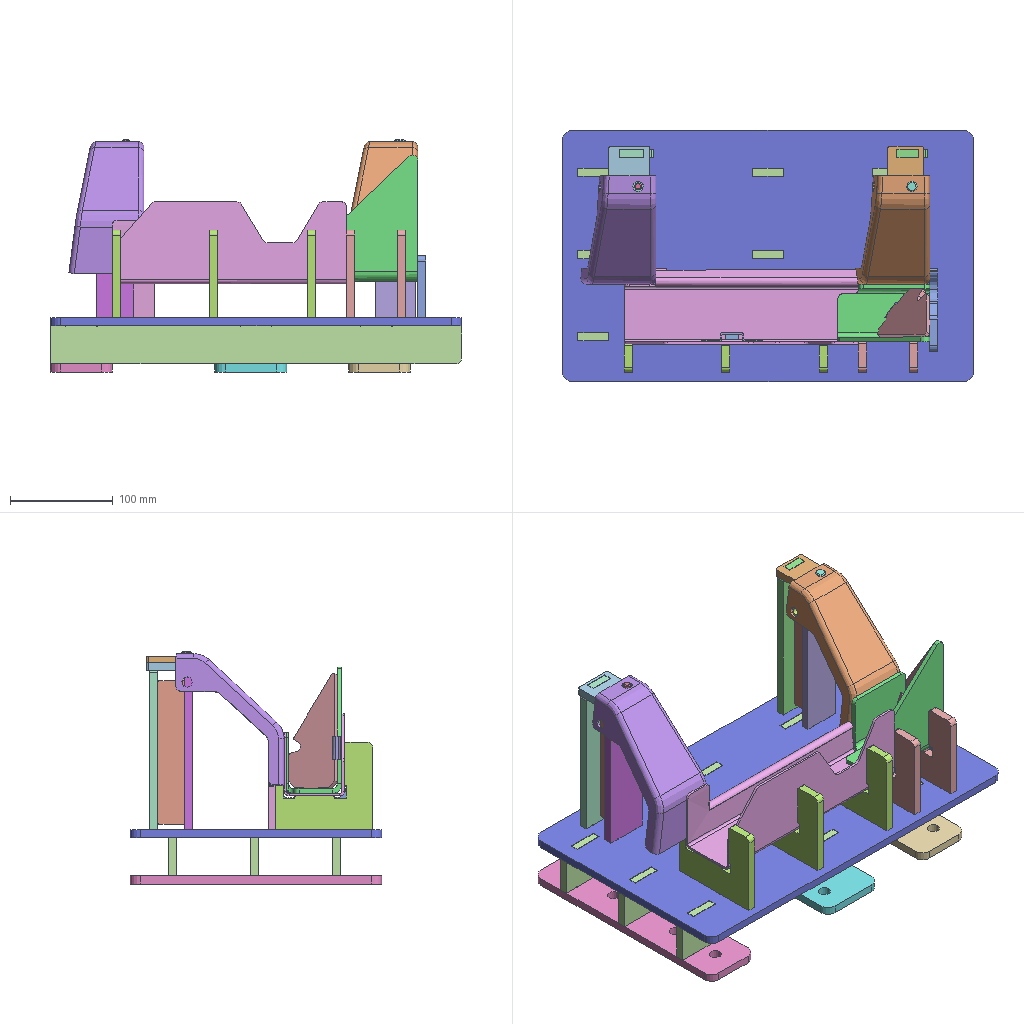Assembly | SolidWorks | 20 different items | 26 placed | box 400 x 245 x 226 mm
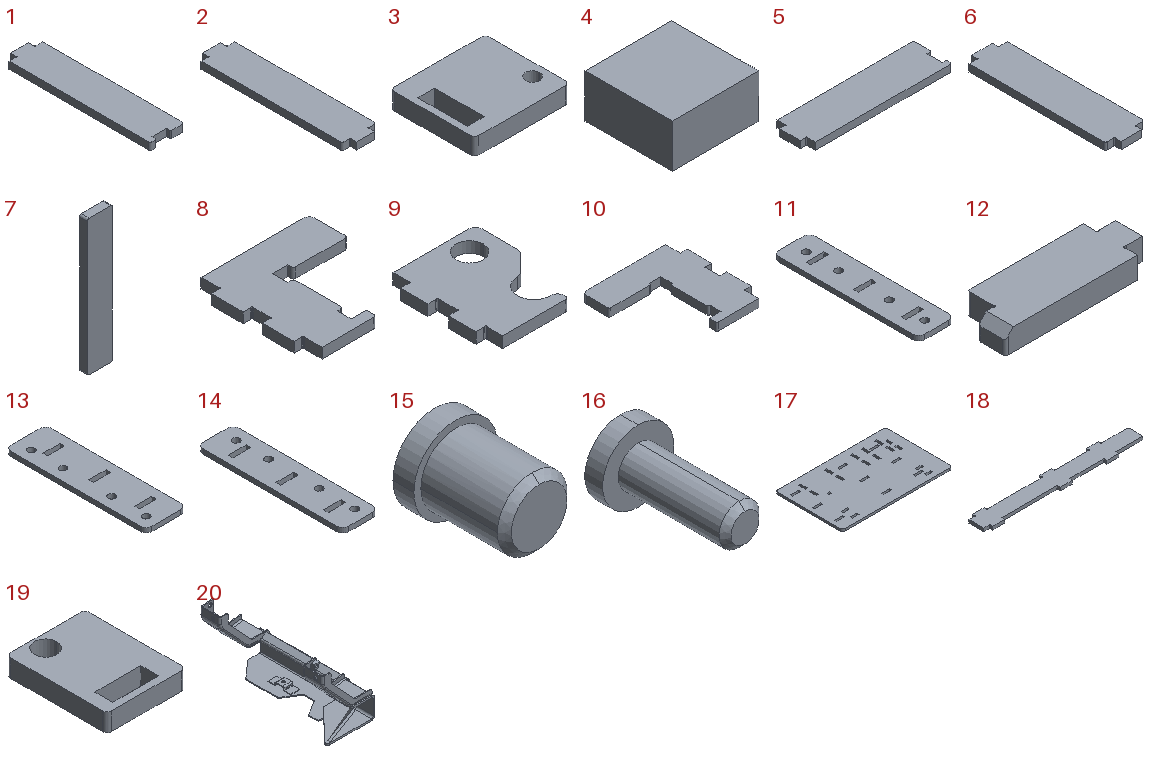Parts list (item | quantity | size | volume | features):
1 | x1 | 38.5 x 167.8 x 8 mm | 49992 mm3 | features Fillet 2, FlatPattern 1, ICE 1, SMBaseFlange 1, SheetMetal 1
2 | x1 | 38.5 x 175.3 x 8 mm | 51881 mm3 | features Fillet 2, FlatPattern 1, ICE 1, SMBaseFlange 1, SheetMetal 1
3 | x1 | 45 x 40 x 8 mm | 12582 mm3 | features Fillet 1, FlatPattern 1, SMBaseFlange 1, SheetMetal 1
4 | x1 | 12 x 12 x 6 mm | 864 mm3 | features FlatPattern 1, SMBaseFlange 1, SheetMetal 1
5 | x1 | 161.8 x 43.5 x 8 mm | 54464 mm3 | features Fillet 2, FlatPattern 1, ICE 1, SMBaseFlange 1, SheetMetal 1
6 | x1 | 43.5 x 169.3 x 8 mm | 56573 mm3 | features Fillet 2, FlatPattern 1, ICE 1, SMBaseFlange 1, SheetMetal 1
7 | x2 | 26 x 8 x 140 mm | 29093 mm3 | features Fillet 1, FlatPattern 1, SMBaseFlange 1, SheetMetal 1
8 | x2 | 92 x 95 x 8 mm | 40763 mm3 | features Fillet 2, FlatPattern 1, ICE 1, SMBaseFlange 1, SheetMetal 1
9 | x1 | 67 x 80 x 8 mm | 31215 mm3 | features Fillet 2, Chamfer 1, FlatPattern 1, ICE 1, SMBaseFlange 1, SheetMetal 1
10 | x3 | 92 x 95 x 8 mm | 39282 mm3 | features Fillet 2, FlatPattern 1, ICE 1, SMBaseFlange 1, SheetMetal 1
11 | x1 | 60 x 245 x 8 mm | 107534 mm3 | features Fillet 1, FlatPattern 1, SMBaseFlange 1, SheetMetal 1
12 | x1 | 55.7 x 20 x 8 mm | 7815 mm3 | features Chamfer 1, Fillet 1, FlatPattern 1, ICE 1, SMBaseFlange 1, SheetMetal 1
13 | x1 | 70 x 245 x 8 mm | 127134 mm3 | features Fillet 1, FlatPattern 1, SMBaseFlange 1, SheetMetal 1
14 | x1 | 60 x 245 x 8 mm | 107534 mm3 | features Fillet 1, FlatPattern 1, SMBaseFlange 1, SheetMetal 1
15 | x1 | 12 x 15 x 12 mm | 1267 mm3 | features Chamfer 1, Revolution 1
16 | x1 | 12 x 21 x 12 mm | 973.861 mm3 | features Chamfer 1, Revolution 1
17 | x1 | 400 x 245 x 8 mm | 741201 mm3 | features FlatPattern 1, SMBaseFlange 1, SheetMetal 1
18 | x3 | 400 x 51.5 x 8 mm | 128767 mm3 | features Fillet 2, FlatPattern 1, ICE 1, SMBaseFlange 1, SheetMetal 1
19 | x1 | 35 x 45 x 8 mm | 10632 mm3 | features Fillet 1, FlatPattern 1, SMBaseFlange 1, SheetMetal 1
20 | x1 | - | - | features ICE 1, MBimport 1
Mates (type | each side: item.copy, entity, surface, feature):
InPlace | 20.1 face plane 2a5-53-11k61_sw0001.stp | 8.1 plane
InPlace | 20.1 face plane 2a5-53-11k61_sw0001.stp | 9.1 plane
InPlace | 20.1 face plane 2a5-53-11k61_sw0001.stp | 10.1 plane
InPlace | 20.1 face plane 2a5-53-11k61_sw0001.stp | 12.1 plane
InPlace | 15.1 plane | assembly plane
InPlace | 15.1 face plane Revolve1 | 19.1 plane
InPlace | 19.1 face plane Base-Flange1 | 1.1 plane
InPlace | 2.1 plane | assembly plane
InPlace | 16.1 plane | assembly plane
InPlace | 20.1 face plane Cut-Extrude1 | 3.1 plane
InPlace | 3.1 face plane Base-Flange1 | 4.1 plane
InPlace | 3.1 face plane Base-Flange1 | 5.1 plane
InPlace | 6.1 plane | assembly plane
Coincident | 1.1 face plane Base-Flange1 | 7.1 face plane Base-Flange1
DistanceDim | 1.1 face plane Base-Flange1 | 7.1 face plane Base-Flange1
DistanceDim | 7.1 face plane Base-Flange1 | 1.1 face plane Base-Flange1
Coincident | 5.1 face plane Base-Flange1 | 7.2 face plane Base-Flange1
DistanceDim | 7.2 face plane Base-Flange1 | 6.1 face plane Base-Flange1
DistanceDim | 5.1 face plane Base-Flange1 | 7.2 face plane Base-Flange1
InPlace | 10.1 face plane Base-Flange1 | 17.1 plane
InPlace | 18.1 plane | assembly plane
InPlace | 18.2 face plane Base-Flange1 | 11.1 plane
InPlace | 18.2 face plane Base-Flange1 | 13.1 plane
InPlace | 18.3 face plane Base-Flange1 | 14.1 plane